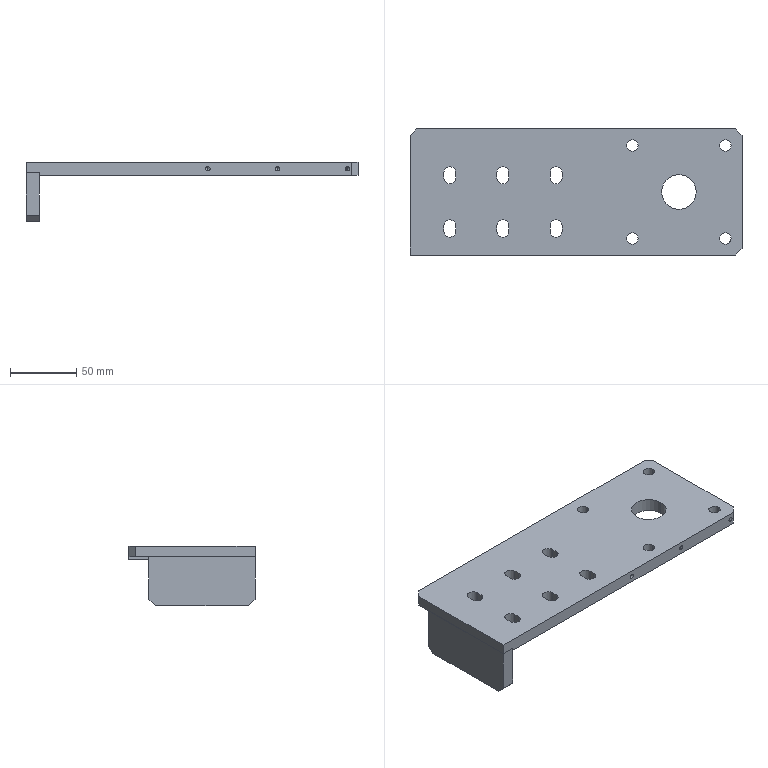Part | SolidWorks | features 3DProfileFeature 4, HoleWzd 4, ICE 4, Chamfer 2, LPattern 2, Extrusion 1 | 2 solids | 65 faces | box 250 x 95 x 45 mm | volume 250777 mm3 | plane 31 | cylinder 28 | cone 6 | commonest cylinder face diameters 9 x12 8.5 x8 3.3 x6 26 x2